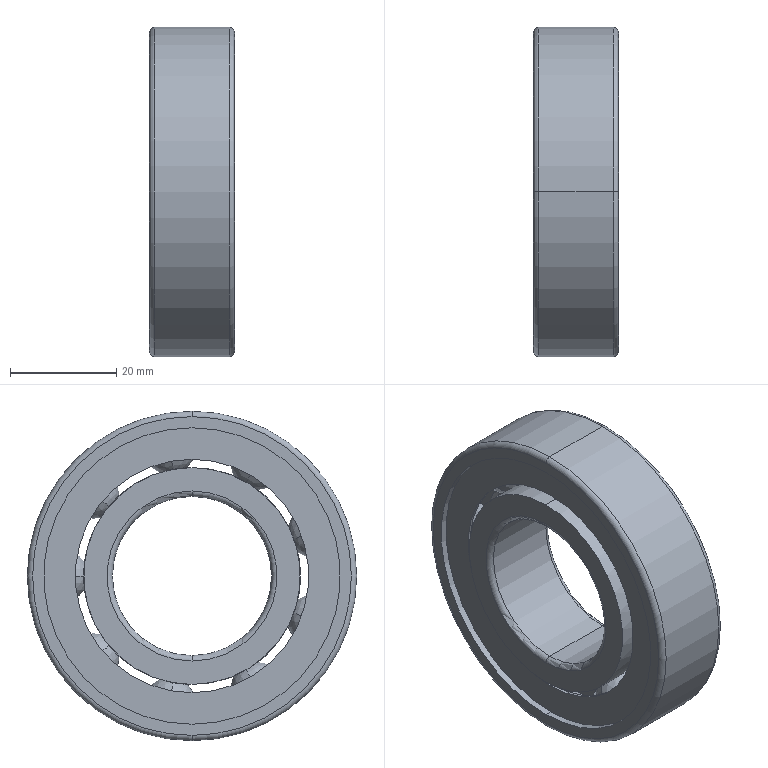Part | STEP file | GB/T276-94 deep groove ball bearing 6206-2Z | 1 solid | 160 faces | box 16 x 62 x 62 mm | volume 23194 mm3 | sphere 72 | torus 38 | plane 26 | cylinder 24 | commonest cylinder face diameters 55.8 x8 40.8 x4 43.943 x4 30 x2 45.681 x2 50.919 x2